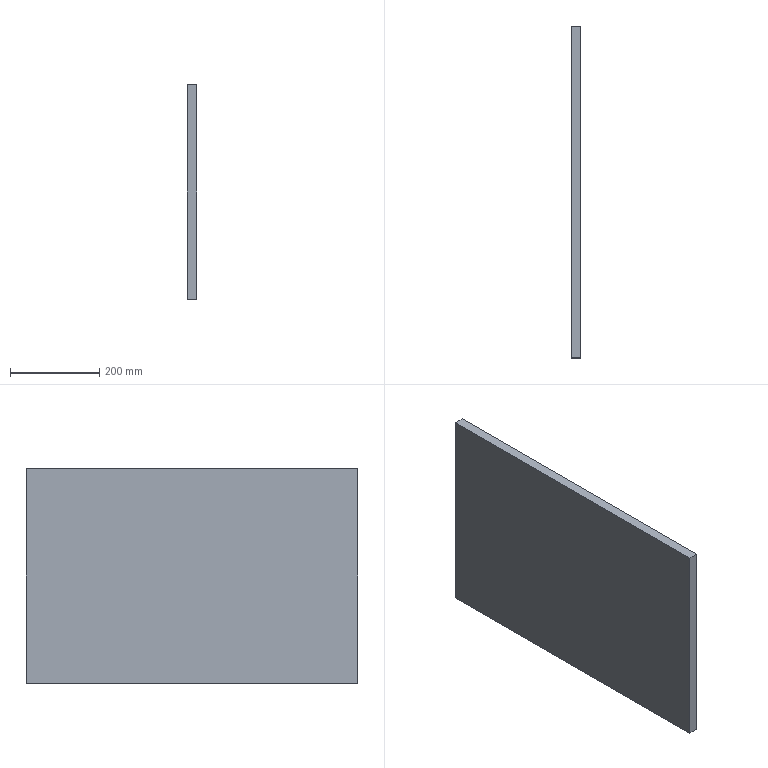Part | NX | features 底座(默认<按焊接>) 2 | 1 solid | 6 faces | box 21.82 x 741.88 x 480 mm | volume 7770154 mm3 | plane 6
STEP:
#1=CARTESIAN_POINT('',(1576.185,763.7,-412.));
#2=VERTEX_POINT('',#1);
#3=CARTESIAN_POINT('',(1554.365,763.7,-412.));
#4=VERTEX_POINT('',#3);
#5=CARTESIAN_POINT('',(1576.185,763.7,-412.));
#6=DIRECTION('',(-1.,0.,0.));
#7=VECTOR('',#6,1000.);
#8=LINE('',#5,#7);
#9=EDGE_CURVE('',#2,#4,#8,.T.);
#10=ORIENTED_EDGE('',*,*,#9,.F.);
#11=CARTESIAN_POINT('',(1576.185,763.7,-892.));
#12=VERTEX_POINT('',#11);
#13=CARTESIAN_POINT('',(1576.185,763.7,-892.));
#14=DIRECTION('',(0.,0.,1.));
#15=VECTOR('',#14,1000.);
#16=LINE('',#13,#15);
#17=EDGE_CURVE('',#12,#2,#16,.T.);
#18=ORIENTED_EDGE('',*,*,#17,.F.);
#19=CARTESIAN_POINT('',(1554.365,763.7,-892.));
#20=VERTEX_POINT('',#19);
#21=CARTESIAN_POINT('',(1576.185,763.7,-892.));
#22=DIRECTION('',(-1.,0.,0.));
#23=VECTOR('',#22,1000.);
#24=LINE('',#21,#23);
#25=EDGE_CURVE('',#12,#20,#24,.T.);
#26=ORIENTED_EDGE('',*,*,#25,.T.);
#27=CARTESIAN_POINT('',(1554.365,763.7,-892.));
#28=DIRECTION('',(0.,0.,1.));
#29=VECTOR('',#28,1000.);
#30=LINE('',#27,#29);
#31=EDGE_CURVE('',#20,#4,#30,.T.);
#32=ORIENTED_EDGE('',*,*,#31,.T.);
#33=EDGE_LOOP('',(#10,#18,#26,#32));
#34=FACE_BOUND('',#33,.T.);
#35=CARTESIAN_POINT('',(1576.185,763.7,-892.));
#36=DIRECTION('',(0.,-1.,0.));
#37=DIRECTION('',(0.,0.,1.));
#38=AXIS2_PLACEMENT_3D('',#35,#36,#37);
#39=PLANE('',#38);
#40=ADVANCED_FACE('',(#34),#39,.F.);
#41=CARTESIAN_POINT('',(1554.365,21.82,-412.));
#42=VERTEX_POINT('',#41);
#43=CARTESIAN_POINT('',(1554.365,763.7,-412.));
#44=DIRECTION('',(0.,-1.,0.));
#45=VECTOR('',#44,1000.);
#46=LINE('',#43,#45);
#47=EDGE_CURVE('',#4,#42,#46,.T.);
#48=ORIENTED_EDGE('',*,*,#47,.F.);
#49=ORIENTED_EDGE('',*,*,#31,.F.);
#50=CARTESIAN_POINT('',(1554.365,21.82,-892.));
#51=VERTEX_POINT('',#50);
#52=CARTESIAN_POINT('',(1554.365,763.7,-892.));
#53=DIRECTION('',(0.,-1.,0.));
#54=VECTOR('',#53,1000.);
#55=LINE('',#52,#54);
#56=EDGE_CURVE('',#20,#51,#55,.T.);
#57=ORIENTED_EDGE('',*,*,#56,.T.);
#58=CARTESIAN_POINT('',(1554.365,21.82,-892.));
#59=DIRECTION('',(0.,0.,1.));
#60=VECTOR('',#59,1000.);
#61=LINE('',#58,#60);
#62=EDGE_CURVE('',#51,#42,#61,.T.);
#63=ORIENTED_EDGE('',*,*,#62,.T.);
#64=EDGE_LOOP('',(#48,#49,#57,#63));
#65=FACE_BOUND('',#64,.T.);
#66=CARTESIAN_POINT('',(1554.365,763.7,-892.));
#67=DIRECTION('',(1.,0.,0.));
#68=DIRECTION('',(0.,0.,1.));
#69=AXIS2_PLACEMENT_3D('',#66,#67,#68);
#70=PLANE('',#69);
#71=ADVANCED_FACE('',(#65),#70,.F.);
#72=CARTESIAN_POINT('',(1576.185,21.82,-412.));
#73=VERTEX_POINT('',#72);
#74=CARTESIAN_POINT('',(1576.185,21.82,-412.));
#75=DIRECTION('',(1.,0.,0.));
#76=VECTOR('',#75,1000.);
#77=LINE('',#74,#76);
#78=EDGE_CURVE('',#42,#73,#77,.T.);
#79=ORIENTED_EDGE('',*,*,#78,.F.);
#80=ORIENTED_EDGE('',*,*,#62,.F.);
#81=CARTESIAN_POINT('',(1576.185,21.82,-892.));
#82=VERTEX_POINT('',#81);
#83=CARTESIAN_POINT('',(1576.185,21.82,-892.));
#84=DIRECTION('',(1.,0.,0.));
#85=VECTOR('',#84,1000.);
#86=LINE('',#83,#85);
#87=EDGE_CURVE('',#51,#82,#86,.T.);
#88=ORIENTED_EDGE('',*,*,#87,.T.);
#89=CARTESIAN_POINT('',(1576.185,21.82,-892.));
#90=DIRECTION('',(0.,0.,1.));
#91=VECTOR('',#90,1000.);
#92=LINE('',#89,#91);
#93=EDGE_CURVE('',#82,#73,#92,.T.);
#94=ORIENTED_EDGE('',*,*,#93,.T.);
#95=EDGE_LOOP('',(#79,#80,#88,#94));
#96=FACE_BOUND('',#95,.T.);
#97=CARTESIAN_POINT('',(1576.185,21.82,-892.));
#98=DIRECTION('',(0.,1.,0.));
#99=DIRECTION('',(-1.,0.,0.));
#100=AXIS2_PLACEMENT_3D('',#97,#98,#99);
#101=PLANE('',#100);
#102=ADVANCED_FACE('',(#96),#101,.F.);
#103=CARTESIAN_POINT('',(1576.185,763.7,-412.));
#104=DIRECTION('',(0.,1.,0.));
#105=VECTOR('',#104,1000.);
#106=LINE('',#103,#105);
#107=EDGE_CURVE('',#73,#2,#106,.T.);
#108=ORIENTED_EDGE('',*,*,#107,.F.);
#109=ORIENTED_EDGE('',*,*,#93,.F.);
#110=CARTESIAN_POINT('',(1576.185,763.7,-892.));
#111=DIRECTION('',(0.,1.,0.));
#112=VECTOR('',#111,1000.);
#113=LINE('',#110,#112);
#114=EDGE_CURVE('',#82,#12,#113,.T.);
#115=ORIENTED_EDGE('',*,*,#114,.T.);
#116=ORIENTED_EDGE('',*,*,#17,.T.);
#117=EDGE_LOOP('',(#108,#109,#115,#116));
#118=FACE_BOUND('',#117,.T.);
#119=CARTESIAN_POINT('',(1576.185,763.7,-892.));
#120=DIRECTION('',(-1.,0.,0.));
#121=DIRECTION('',(0.,-1.,0.));
#122=AXIS2_PLACEMENT_3D('',#119,#120,#121);
#123=PLANE('',#122);
#124=ADVANCED_FACE('',(#118),#123,.F.);
#125=ORIENTED_EDGE('',*,*,#25,.F.);
#126=ORIENTED_EDGE('',*,*,#114,.F.);
#127=ORIENTED_EDGE('',*,*,#87,.F.);
#128=ORIENTED_EDGE('',*,*,#56,.F.);
#129=EDGE_LOOP('',(#125,#126,#127,#128));
#130=FACE_BOUND('',#129,.T.);
#131=CARTESIAN_POINT('',(1554.365,763.7,-892.));
#132=DIRECTION('',(0.,0.,-1.));
#133=DIRECTION('',(1.,0.,0.));
#134=AXIS2_PLACEMENT_3D('',#131,#132,#133);
#135=PLANE('',#134);
#136=ADVANCED_FACE('',(#130),#135,.T.);
#137=ORIENTED_EDGE('',*,*,#9,.T.);
#138=ORIENTED_EDGE('',*,*,#47,.T.);
#139=ORIENTED_EDGE('',*,*,#78,.T.);
#140=ORIENTED_EDGE('',*,*,#107,.T.);
#141=EDGE_LOOP('',(#137,#138,#139,#140));
#142=FACE_BOUND('',#141,.T.);
#143=CARTESIAN_POINT('',(1554.365,763.7,-412.));
#144=DIRECTION('',(0.,0.,-1.));
#145=DIRECTION('',(1.,0.,0.));
#146=AXIS2_PLACEMENT_3D('',#143,#144,#145);
#147=PLANE('',#146);
#148=ADVANCED_FACE('',(#142),#147,.F.);
#149=CLOSED_SHELL('',(#40,#71,#102,#124,#136,#148));
#150=MANIFOLD_SOLID_BREP('',#149);
#151=(LENGTH_UNIT()NAMED_UNIT(*)SI_UNIT(.MILLI.,.METRE.));
#152=UNCERTAINTY_MEASURE_WITH_UNIT(LENGTH_MEASURE(0.00001),#151,'','');
#153=(NAMED_UNIT(*)PLANE_ANGLE_UNIT()SI_UNIT($,.RADIAN.));
#154=(NAMED_UNIT(*)SI_UNIT($,.STERADIAN.)SOLID_ANGLE_UNIT());
#155=(GEOMETRIC_REPRESENTATION_CONTEXT(3)GLOBAL_UNCERTAINTY_ASSIGNED_CONTEXT((#152))GLOBAL_UNIT_ASSIGNED_CONTEXT((#151,#153,#154))REPRESENTATION_CONTEXT('',''));
#156=ADVANCED_BREP_SHAPE_REPRESENTATION('',(#150),#155);